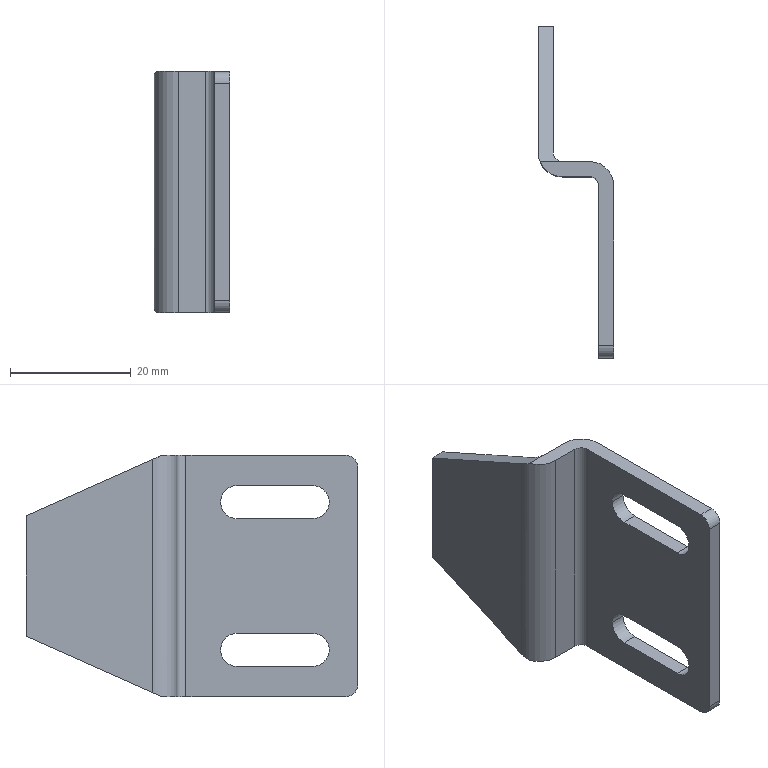Part | NX | features BREP 1 | 1 solid | 28 faces | box 12.5 x 55 x 40 mm | volume 5235 mm3 | plane 16 | cylinder 12 | commonest cylinder face diameters 5.5 x6 3 x2 4 x2 8 x2
STEP:
#1=CARTESIAN_POINT('',(0.,-7.25,-12.25));
#2=VERTEX_POINT('',#1);
#3=CARTESIAN_POINT('',(0.,-10.,-9.5));
#4=VERTEX_POINT('',#3);
#5=CARTESIAN_POINT('',(0.,-10.,-12.25));
#6=DIRECTION('',(1.,0.,0.));
#7=DIRECTION('',(0.,1.,0.));
#8=AXIS2_PLACEMENT_3D('',#5,#6,#7);
#9=CIRCLE('',#8,2.75);
#10=EDGE_CURVE('',#2,#4,#9,.T.);
#11=ORIENTED_EDGE('',*,*,#10,.F.);
#12=CARTESIAN_POINT('',(2.5,-7.25,-12.25));
#13=VERTEX_POINT('',#12);
#14=CARTESIAN_POINT('',(-10.,-7.25,-12.25));
#15=DIRECTION('',(1.,0.,0.));
#16=VECTOR('',#15,1000.);
#17=LINE('',#14,#16);
#18=EDGE_CURVE('',#2,#13,#17,.T.);
#19=ORIENTED_EDGE('',*,*,#18,.T.);
#20=CARTESIAN_POINT('',(2.5,-10.,-9.5));
#21=VERTEX_POINT('',#20);
#22=CARTESIAN_POINT('',(2.5,-10.,-12.25));
#23=DIRECTION('',(1.,0.,0.));
#24=DIRECTION('',(0.,-1.,0.));
#25=AXIS2_PLACEMENT_3D('',#22,#23,#24);
#26=CIRCLE('',#25,2.75);
#27=EDGE_CURVE('',#13,#21,#26,.T.);
#28=ORIENTED_EDGE('',*,*,#27,.T.);
#29=CARTESIAN_POINT('',(-10.,-10.,-9.5));
#30=DIRECTION('',(1.,0.,0.));
#31=VECTOR('',#30,1000.);
#32=LINE('',#29,#31);
#33=EDGE_CURVE('',#4,#21,#32,.T.);
#34=ORIENTED_EDGE('',*,*,#33,.F.);
#35=EDGE_LOOP('',(#11,#19,#28,#34));
#36=FACE_BOUND('',#35,.T.);
#37=CARTESIAN_POINT('',(-10.,-10.,-12.25));
#38=DIRECTION('',(1.,0.,0.));
#39=DIRECTION('',(0.,1.,0.));
#40=AXIS2_PLACEMENT_3D('',#37,#38,#39);
#41=CYLINDRICAL_SURFACE('',#40,2.75);
#42=ADVANCED_FACE('',(#36),#41,.F.);
#43=CARTESIAN_POINT('',(0.,-7.25,12.25));
#44=VERTEX_POINT('',#43);
#45=CARTESIAN_POINT('',(0.,-10.,15.));
#46=VERTEX_POINT('',#45);
#47=CARTESIAN_POINT('',(0.,-10.,12.25));
#48=DIRECTION('',(1.,0.,0.));
#49=DIRECTION('',(0.,1.,0.));
#50=AXIS2_PLACEMENT_3D('',#47,#48,#49);
#51=CIRCLE('',#50,2.75);
#52=EDGE_CURVE('',#44,#46,#51,.T.);
#53=ORIENTED_EDGE('',*,*,#52,.F.);
#54=CARTESIAN_POINT('',(2.5,-7.25,12.25));
#55=VERTEX_POINT('',#54);
#56=CARTESIAN_POINT('',(-10.,-7.25,12.25));
#57=DIRECTION('',(1.,0.,0.));
#58=VECTOR('',#57,1000.);
#59=LINE('',#56,#58);
#60=EDGE_CURVE('',#44,#55,#59,.T.);
#61=ORIENTED_EDGE('',*,*,#60,.T.);
#62=CARTESIAN_POINT('',(2.5,-10.,15.));
#63=VERTEX_POINT('',#62);
#64=CARTESIAN_POINT('',(2.5,-10.,12.25));
#65=DIRECTION('',(1.,0.,0.));
#66=DIRECTION('',(0.,1.,0.));
#67=AXIS2_PLACEMENT_3D('',#64,#65,#66);
#68=CIRCLE('',#67,2.75);
#69=EDGE_CURVE('',#55,#63,#68,.T.);
#70=ORIENTED_EDGE('',*,*,#69,.T.);
#71=CARTESIAN_POINT('',(-10.,-10.,15.));
#72=DIRECTION('',(1.,0.,0.));
#73=VECTOR('',#72,1000.);
#74=LINE('',#71,#73);
#75=EDGE_CURVE('',#46,#63,#74,.T.);
#76=ORIENTED_EDGE('',*,*,#75,.F.);
#77=EDGE_LOOP('',(#53,#61,#70,#76));
#78=FACE_BOUND('',#77,.T.);
#79=CARTESIAN_POINT('',(-10.,-10.,12.25));
#80=DIRECTION('',(1.,0.,0.));
#81=DIRECTION('',(0.,1.,0.));
#82=AXIS2_PLACEMENT_3D('',#79,#80,#81);
#83=CYLINDRICAL_SURFACE('',#82,2.75);
#84=ADVANCED_FACE('',(#78),#83,.F.);
#85=CARTESIAN_POINT('',(2.5,-30.,18.));
#86=VERTEX_POINT('',#85);
#87=CARTESIAN_POINT('',(2.5,-30.,-18.));
#88=VERTEX_POINT('',#87);
#89=CARTESIAN_POINT('',(2.5,-30.,20.));
#90=DIRECTION('',(0.,0.,-1.));
#91=VECTOR('',#90,1000.);
#92=LINE('',#89,#91);
#93=EDGE_CURVE('',#86,#88,#92,.T.);
#94=ORIENTED_EDGE('',*,*,#93,.T.);
#95=CARTESIAN_POINT('',(2.5,-28.,-20.));
#96=VERTEX_POINT('',#95);
#97=CARTESIAN_POINT('',(2.5,-28.,-18.));
#98=DIRECTION('',(1.,0.,0.));
#99=DIRECTION('',(0.,-1.,0.));
#100=AXIS2_PLACEMENT_3D('',#97,#98,#99);
#101=CIRCLE('',#100,2.);
#102=EDGE_CURVE('',#88,#96,#101,.T.);
#103=ORIENTED_EDGE('',*,*,#102,.T.);
#104=CARTESIAN_POINT('',(2.5,-1.5,-20.));
#105=VERTEX_POINT('',#104);
#106=CARTESIAN_POINT('',(2.5,2.5,-20.));
#107=DIRECTION('',(0.,1.,0.));
#108=VECTOR('',#107,1000.);
#109=LINE('',#106,#108);
#110=EDGE_CURVE('',#96,#105,#109,.T.);
#111=ORIENTED_EDGE('',*,*,#110,.T.);
#112=CARTESIAN_POINT('',(2.5,-1.5,20.));
#113=VERTEX_POINT('',#112);
#114=CARTESIAN_POINT('',(2.5,-1.5,20.));
#115=DIRECTION('',(0.,0.,1.));
#116=VECTOR('',#115,1000.);
#117=LINE('',#114,#116);
#118=EDGE_CURVE('',#105,#113,#117,.T.);
#119=ORIENTED_EDGE('',*,*,#118,.T.);
#120=CARTESIAN_POINT('',(2.5,-28.,20.));
#121=VERTEX_POINT('',#120);
#122=CARTESIAN_POINT('',(2.5,2.5,20.));
#123=DIRECTION('',(0.,1.,0.));
#124=VECTOR('',#123,1000.);
#125=LINE('',#122,#124);
#126=EDGE_CURVE('',#121,#113,#125,.T.);
#127=ORIENTED_EDGE('',*,*,#126,.F.);
#128=CARTESIAN_POINT('',(2.5,-28.,18.));
#129=DIRECTION('',(1.,0.,0.));
#130=DIRECTION('',(0.,-1.,0.));
#131=AXIS2_PLACEMENT_3D('',#128,#129,#130);
#132=CIRCLE('',#131,2.);
#133=EDGE_CURVE('',#121,#86,#132,.T.);
#134=ORIENTED_EDGE('',*,*,#133,.T.);
#135=EDGE_LOOP('',(#94,#103,#111,#119,#127,#134));
#136=FACE_BOUND('',#135,.T.);
#137=CARTESIAN_POINT('',(2.5,-22.5,-9.5));
#138=VERTEX_POINT('',#137);
#139=CARTESIAN_POINT('',(2.5,-10.,-9.5));
#140=DIRECTION('',(0.,-1.,0.));
#141=VECTOR('',#140,1000.);
#142=LINE('',#139,#141);
#143=EDGE_CURVE('',#21,#138,#142,.T.);
#144=ORIENTED_EDGE('',*,*,#143,.F.);
#145=ORIENTED_EDGE('',*,*,#27,.F.);
#146=CARTESIAN_POINT('',(2.5,-10.,-15.));
#147=VERTEX_POINT('',#146);
#148=CARTESIAN_POINT('',(2.5,-10.,-12.25));
#149=DIRECTION('',(1.,0.,0.));
#150=DIRECTION('',(0.,-1.,0.));
#151=AXIS2_PLACEMENT_3D('',#148,#149,#150);
#152=CIRCLE('',#151,2.75);
#153=EDGE_CURVE('',#147,#13,#152,.T.);
#154=ORIENTED_EDGE('',*,*,#153,.F.);
#155=CARTESIAN_POINT('',(2.5,-22.5,-15.));
#156=VERTEX_POINT('',#155);
#157=CARTESIAN_POINT('',(2.5,-10.,-15.));
#158=DIRECTION('',(0.,1.,0.));
#159=VECTOR('',#158,1000.);
#160=LINE('',#157,#159);
#161=EDGE_CURVE('',#156,#147,#160,.T.);
#162=ORIENTED_EDGE('',*,*,#161,.F.);
#163=CARTESIAN_POINT('',(2.5,-22.5,-12.25));
#164=DIRECTION('',(1.,0.,0.));
#165=DIRECTION('',(0.,-1.,0.));
#166=AXIS2_PLACEMENT_3D('',#163,#164,#165);
#167=CIRCLE('',#166,2.75);
#168=EDGE_CURVE('',#138,#156,#167,.T.);
#169=ORIENTED_EDGE('',*,*,#168,.F.);
#170=EDGE_LOOP('',(#144,#145,#154,#162,#169));
#171=FACE_BOUND('',#170,.T.);
#172=CARTESIAN_POINT('',(2.5,-22.5,15.));
#173=VERTEX_POINT('',#172);
#174=CARTESIAN_POINT('',(2.5,-10.,15.));
#175=DIRECTION('',(0.,-1.,0.));
#176=VECTOR('',#175,1000.);
#177=LINE('',#174,#176);
#178=EDGE_CURVE('',#63,#173,#177,.T.);
#179=ORIENTED_EDGE('',*,*,#178,.F.);
#180=ORIENTED_EDGE('',*,*,#69,.F.);
#181=CARTESIAN_POINT('',(2.5,-10.,9.5));
#182=VERTEX_POINT('',#181);
#183=CARTESIAN_POINT('',(2.5,-10.,12.25));
#184=DIRECTION('',(1.,0.,0.));
#185=DIRECTION('',(0.,1.,0.));
#186=AXIS2_PLACEMENT_3D('',#183,#184,#185);
#187=CIRCLE('',#186,2.75);
#188=EDGE_CURVE('',#182,#55,#187,.T.);
#189=ORIENTED_EDGE('',*,*,#188,.F.);
#190=CARTESIAN_POINT('',(2.5,-22.5,9.5));
#191=VERTEX_POINT('',#190);
#192=CARTESIAN_POINT('',(2.5,-10.,9.5));
#193=DIRECTION('',(0.,1.,0.));
#194=VECTOR('',#193,1000.);
#195=LINE('',#192,#194);
#196=EDGE_CURVE('',#191,#182,#195,.T.);
#197=ORIENTED_EDGE('',*,*,#196,.F.);
#198=CARTESIAN_POINT('',(2.5,-22.5,12.25));
#199=DIRECTION('',(1.,0.,0.));
#200=DIRECTION('',(0.,1.,0.));
#201=AXIS2_PLACEMENT_3D('',#198,#199,#200);
#202=CIRCLE('',#201,2.75);
#203=EDGE_CURVE('',#173,#191,#202,.T.);
#204=ORIENTED_EDGE('',*,*,#203,.F.);
#205=EDGE_LOOP('',(#179,#180,#189,#197,#204));
#206=FACE_BOUND('',#205,.T.);
#207=CARTESIAN_POINT('',(2.5,2.5,20.));
#208=DIRECTION('',(-1.,0.,0.));
#209=DIRECTION('',(0.,1.,0.));
#210=AXIS2_PLACEMENT_3D('',#207,#208,#209);
#211=PLANE('',#210);
#212=ADVANCED_FACE('',(#136,#171,#206),#211,.F.);
#213=CARTESIAN_POINT('',(-1.5,2.5,20.));
#214=VERTEX_POINT('',#213);
#215=CARTESIAN_POINT('',(-6.,2.5,20.));
#216=VERTEX_POINT('',#215);
#217=CARTESIAN_POINT('',(-7.5,2.5,20.));
#218=DIRECTION('',(-1.,0.,0.));
#219=VECTOR('',#218,1000.);
#220=LINE('',#217,#219);
#221=EDGE_CURVE('',#214,#216,#220,.T.);
#222=ORIENTED_EDGE('',*,*,#221,.F.);
#223=CARTESIAN_POINT('',(-1.5,2.5,-20.));
#224=VERTEX_POINT('',#223);
#225=CARTESIAN_POINT('',(-1.5,2.5,20.));
#226=DIRECTION('',(0.,0.,-1.));
#227=VECTOR('',#226,1000.);
#228=LINE('',#225,#227);
#229=EDGE_CURVE('',#214,#224,#228,.T.);
#230=ORIENTED_EDGE('',*,*,#229,.T.);
#231=CARTESIAN_POINT('',(-6.,2.5,-20.));
#232=VERTEX_POINT('',#231);
#233=CARTESIAN_POINT('',(-7.5,2.5,-20.));
#234=DIRECTION('',(-1.,0.,0.));
#235=VECTOR('',#234,1000.);
#236=LINE('',#233,#235);
#237=EDGE_CURVE('',#224,#232,#236,.T.);
#238=ORIENTED_EDGE('',*,*,#237,.T.);
#239=CARTESIAN_POINT('',(-6.,2.5,20.));
#240=DIRECTION('',(0.,0.,1.));
#241=VECTOR('',#240,1000.);
#242=LINE('',#239,#241);
#243=EDGE_CURVE('',#232,#216,#242,.T.);
#244=ORIENTED_EDGE('',*,*,#243,.T.);
#245=EDGE_LOOP('',(#222,#230,#238,#244));
#246=FACE_BOUND('',#245,.T.);
#247=CARTESIAN_POINT('',(-7.5,2.5,20.));
#248=DIRECTION('',(0.,-1.,0.));
#249=DIRECTION('',(0.,0.,-1.));
#250=AXIS2_PLACEMENT_3D('',#247,#248,#249);
#251=PLANE('',#250);
#252=ADVANCED_FACE('',(#246),#251,.F.);
#253=CARTESIAN_POINT('',(-7.5,25.,10.));
#254=VERTEX_POINT('',#253);
#255=CARTESIAN_POINT('',(-7.5,4.,19.333));
#256=VERTEX_POINT('',#255);
#257=CARTESIAN_POINT('',(-7.5,21.289,11.649));
#258=DIRECTION('',(0.,-0.9138,0.4061));
#259=VECTOR('',#258,1000.);
#260=LINE('',#257,#259);
#261=EDGE_CURVE('',#254,#256,#260,.T.);
#262=ORIENTED_EDGE('',*,*,#261,.T.);
#263=CARTESIAN_POINT('',(-7.5,4.,-19.333));
#264=VERTEX_POINT('',#263);
#265=CARTESIAN_POINT('',(-7.5,4.,-20.));
#266=DIRECTION('',(0.,0.,-1.));
#267=VECTOR('',#266,1000.);
#268=LINE('',#265,#267);
#269=EDGE_CURVE('',#256,#264,#268,.T.);
#270=ORIENTED_EDGE('',*,*,#269,.T.);
#271=CARTESIAN_POINT('',(-7.5,25.,-10.));
#272=VERTEX_POINT('',#271);
#273=CARTESIAN_POINT('',(-7.5,36.134,-5.052));
#274=DIRECTION('',(0.,0.9138,0.4061));
#275=VECTOR('',#274,1000.);
#276=LINE('',#273,#275);
#277=EDGE_CURVE('',#264,#272,#276,.T.);
#278=ORIENTED_EDGE('',*,*,#277,.T.);
#279=CARTESIAN_POINT('',(-7.5,25.,20.));
#280=DIRECTION('',(0.,0.,-1.));
#281=VECTOR('',#280,1000.);
#282=LINE('',#279,#281);
#283=EDGE_CURVE('',#254,#272,#282,.T.);
#284=ORIENTED_EDGE('',*,*,#283,.F.);
#285=EDGE_LOOP('',(#262,#270,#278,#284));
#286=FACE_BOUND('',#285,.T.);
#287=CARTESIAN_POINT('',(-7.5,25.,20.));
#288=DIRECTION('',(-1.,0.,0.));
#289=DIRECTION('',(0.,1.,0.));
#290=AXIS2_PLACEMENT_3D('',#287,#288,#289);
#291=PLANE('',#290);
#292=ADVANCED_FACE('',(#286),#291,.F.);
#293=ORIENTED_EDGE('',*,*,#283,.T.);
#294=CARTESIAN_POINT('',(-10.,25.,-10.));
#295=VERTEX_POINT('',#294);
#296=CARTESIAN_POINT('',(-10.,25.,-10.));
#297=DIRECTION('',(1.,0.,0.));
#298=VECTOR('',#297,1000.);
#299=LINE('',#296,#298);
#300=EDGE_CURVE('',#295,#272,#299,.T.);
#301=ORIENTED_EDGE('',*,*,#300,.F.);
#302=CARTESIAN_POINT('',(-10.,25.,10.));
#303=VERTEX_POINT('',#302);
#304=CARTESIAN_POINT('',(-10.,25.,20.));
#305=DIRECTION('',(0.,0.,-1.));
#306=VECTOR('',#305,1000.);
#307=LINE('',#304,#306);
#308=EDGE_CURVE('',#303,#295,#307,.T.);
#309=ORIENTED_EDGE('',*,*,#308,.F.);
#310=CARTESIAN_POINT('',(-10.,25.,10.));
#311=DIRECTION('',(1.,0.,0.));
#312=VECTOR('',#311,1000.);
#313=LINE('',#310,#312);
#314=EDGE_CURVE('',#303,#254,#313,.T.);
#315=ORIENTED_EDGE('',*,*,#314,.T.);
#316=EDGE_LOOP('',(#293,#301,#309,#315));
#317=FACE_BOUND('',#316,.T.);
#318=CARTESIAN_POINT('',(-10.,25.,20.));
#319=DIRECTION('',(0.,-1.,0.));
#320=DIRECTION('',(0.,0.,-1.));
#321=AXIS2_PLACEMENT_3D('',#318,#319,#320);
#322=PLANE('',#321);
#323=ADVANCED_FACE('',(#317),#322,.F.);
#324=CARTESIAN_POINT('',(-10.,4.,-19.333));
#325=VERTEX_POINT('',#324);
#326=CARTESIAN_POINT('',(-10.,25.,-10.));
#327=DIRECTION('',(0.,-0.9138,-0.4061));
#328=VECTOR('',#327,1000.);
#329=LINE('',#326,#328);
#330=EDGE_CURVE('',#295,#325,#329,.T.);
#331=ORIENTED_EDGE('',*,*,#330,.T.);
#332=CARTESIAN_POINT('',(-10.,4.,19.333));
#333=VERTEX_POINT('',#332);
#334=CARTESIAN_POINT('',(-10.,4.,20.));
#335=DIRECTION('',(0.,0.,1.));
#336=VECTOR('',#335,1000.);
#337=LINE('',#334,#336);
#338=EDGE_CURVE('',#325,#333,#337,.T.);
#339=ORIENTED_EDGE('',*,*,#338,.T.);
#340=CARTESIAN_POINT('',(-10.,25.,10.));
#341=DIRECTION('',(0.,0.9138,-0.4061));
#342=VECTOR('',#341,1000.);
#343=LINE('',#340,#342);
#344=EDGE_CURVE('',#333,#303,#343,.T.);
#345=ORIENTED_EDGE('',*,*,#344,.T.);
#346=ORIENTED_EDGE('',*,*,#308,.T.);
#347=EDGE_LOOP('',(#331,#339,#345,#346));
#348=FACE_BOUND('',#347,.T.);
#349=CARTESIAN_POINT('',(-10.,0.,20.));
#350=DIRECTION('',(1.,0.,0.));
#351=DIRECTION('',(0.,1.,0.));
#352=AXIS2_PLACEMENT_3D('',#349,#350,#351);
#353=PLANE('',#352);
#354=ADVANCED_FACE('',(#348),#353,.F.);
#355=CARTESIAN_POINT('',(-6.,0.,20.));
#356=VERTEX_POINT('',#355);
#357=CARTESIAN_POINT('',(-1.5,0.,20.));
#358=VERTEX_POINT('',#357);
#359=CARTESIAN_POINT('',(0.,0.,20.));
#360=DIRECTION('',(1.,0.,0.));
#361=VECTOR('',#360,1000.);
#362=LINE('',#359,#361);
#363=EDGE_CURVE('',#356,#358,#362,.T.);
#364=ORIENTED_EDGE('',*,*,#363,.F.);
#365=CARTESIAN_POINT('',(-6.,0.,-20.));
#366=VERTEX_POINT('',#365);
#367=CARTESIAN_POINT('',(-6.,0.,20.));
#368=DIRECTION('',(0.,0.,-1.));
#369=VECTOR('',#368,1000.);
#370=LINE('',#367,#369);
#371=EDGE_CURVE('',#356,#366,#370,.T.);
#372=ORIENTED_EDGE('',*,*,#371,.T.);
#373=CARTESIAN_POINT('',(-1.5,0.,-20.));
#374=VERTEX_POINT('',#373);
#375=CARTESIAN_POINT('',(0.,0.,-20.));
#376=DIRECTION('',(1.,0.,0.));
#377=VECTOR('',#376,1000.);
#378=LINE('',#375,#377);
#379=EDGE_CURVE('',#366,#374,#378,.T.);
#380=ORIENTED_EDGE('',*,*,#379,.T.);
#381=CARTESIAN_POINT('',(-1.5,0.,20.));
#382=DIRECTION('',(0.,0.,1.));
#383=VECTOR('',#382,1000.);
#384=LINE('',#381,#383);
#385=EDGE_CURVE('',#374,#358,#384,.T.);
#386=ORIENTED_EDGE('',*,*,#385,.T.);
#387=EDGE_LOOP('',(#364,#372,#380,#386));
#388=FACE_BOUND('',#387,.T.);
#389=CARTESIAN_POINT('',(0.,0.,20.));
#390=DIRECTION('',(0.,1.,0.));
#391=DIRECTION('',(1.,0.,0.));
#392=AXIS2_PLACEMENT_3D('',#389,#390,#391);
#393=PLANE('',#392);
#394=ADVANCED_FACE('',(#388),#393,.F.);
#395=CARTESIAN_POINT('',(0.,-1.5,-20.));
#396=VERTEX_POINT('',#395);
#397=CARTESIAN_POINT('',(0.,-28.,-20.));
#398=VERTEX_POINT('',#397);
#399=CARTESIAN_POINT('',(0.,-30.,-20.));
#400=DIRECTION('',(0.,-1.,0.));
#401=VECTOR('',#400,1000.);
#402=LINE('',#399,#401);
#403=EDGE_CURVE('',#396,#398,#402,.T.);
#404=ORIENTED_EDGE('',*,*,#403,.T.);
#405=CARTESIAN_POINT('',(0.,-30.,-18.));
#406=VERTEX_POINT('',#405);
#407=CARTESIAN_POINT('',(0.,-28.,-18.));
#408=DIRECTION('',(-1.,0.,0.));
#409=DIRECTION('',(0.,1.,0.));
#410=AXIS2_PLACEMENT_3D('',#407,#408,#409);
#411=CIRCLE('',#410,2.);
#412=EDGE_CURVE('',#398,#406,#411,.T.);
#413=ORIENTED_EDGE('',*,*,#412,.T.);
#414=CARTESIAN_POINT('',(0.,-30.,18.));
#415=VERTEX_POINT('',#414);
#416=CARTESIAN_POINT('',(0.,-30.,20.));
#417=DIRECTION('',(0.,0.,-1.));
#418=VECTOR('',#417,1000.);
#419=LINE('',#416,#418);
#420=EDGE_CURVE('',#415,#406,#419,.T.);
#421=ORIENTED_EDGE('',*,*,#420,.F.);
#422=CARTESIAN_POINT('',(0.,-28.,20.));
#423=VERTEX_POINT('',#422);
#424=CARTESIAN_POINT('',(0.,-28.,18.));
#425=DIRECTION('',(-1.,0.,0.));
#426=DIRECTION('',(0.,1.,0.));
#427=AXIS2_PLACEMENT_3D('',#424,#425,#426);
#428=CIRCLE('',#427,2.);
#429=EDGE_CURVE('',#415,#423,#428,.T.);
#430=ORIENTED_EDGE('',*,*,#429,.T.);
#431=CARTESIAN_POINT('',(0.,-1.5,20.));
#432=VERTEX_POINT('',#431);
#433=CARTESIAN_POINT('',(0.,-30.,20.));
#434=DIRECTION('',(0.,-1.,0.));
#435=VECTOR('',#434,1000.);
#436=LINE('',#433,#435);
#437=EDGE_CURVE('',#432,#423,#436,.T.);
#438=ORIENTED_EDGE('',*,*,#437,.F.);
#439=CARTESIAN_POINT('',(0.,-1.5,-20.));
#440=DIRECTION('',(0.,0.,-1.));
#441=VECTOR('',#440,1000.);
#442=LINE('',#439,#441);
#443=EDGE_CURVE('',#432,#396,#442,.T.);
#444=ORIENTED_EDGE('',*,*,#443,.T.);
#445=EDGE_LOOP('',(#404,#413,#421,#430,#438,#444));
#446=FACE_BOUND('',#445,.T.);
#447=CARTESIAN_POINT('',(0.,-22.5,-15.));
#448=VERTEX_POINT('',#447);
#449=CARTESIAN_POINT('',(0.,-10.,-15.));
#450=VERTEX_POINT('',#449);
#451=CARTESIAN_POINT('',(0.,-30.,-15.));
#452=DIRECTION('',(0.,1.,0.));
#453=VECTOR('',#452,1000.);
#454=LINE('',#451,#453);
#455=EDGE_CURVE('',#448,#450,#454,.T.);
#456=ORIENTED_EDGE('',*,*,#455,.T.);
#457=CARTESIAN_POINT('',(0.,-10.,-12.25));
#458=DIRECTION('',(1.,0.,0.));
#459=DIRECTION('',(0.,1.,0.));
#460=AXIS2_PLACEMENT_3D('',#457,#458,#459);
#461=CIRCLE('',#460,2.75);
#462=EDGE_CURVE('',#450,#2,#461,.T.);
#463=ORIENTED_EDGE('',*,*,#462,.T.);
#464=ORIENTED_EDGE('',*,*,#10,.T.);
#465=CARTESIAN_POINT('',(0.,-22.5,-9.5));
#466=VERTEX_POINT('',#465);
#467=CARTESIAN_POINT('',(0.,-30.,-9.5));
#468=DIRECTION('',(0.,-1.,0.));
#469=VECTOR('',#468,1000.);
#470=LINE('',#467,#469);
#471=EDGE_CURVE('',#4,#466,#470,.T.);
#472=ORIENTED_EDGE('',*,*,#471,.T.);
#473=CARTESIAN_POINT('',(0.,-22.5,-12.25));
#474=DIRECTION('',(1.,0.,0.));
#475=DIRECTION('',(0.,1.,0.));
#476=AXIS2_PLACEMENT_3D('',#473,#474,#475);
#477=CIRCLE('',#476,2.75);
#478=EDGE_CURVE('',#466,#448,#477,.T.);
#479=ORIENTED_EDGE('',*,*,#478,.T.);
#480=EDGE_LOOP('',(#456,#463,#464,#472,#479));
#481=FACE_BOUND('',#480,.T.);
#482=CARTESIAN_POINT('',(0.,-22.5,9.5));
#483=VERTEX_POINT('',#482);
#484=CARTESIAN_POINT('',(0.,-10.,9.5));
#485=VERTEX_POINT('',#484);
#486=CARTESIAN_POINT('',(0.,-30.,9.5));
#487=DIRECTION('',(0.,1.,0.));
#488=VECTOR('',#487,1000.);
#489=LINE('',#486,#488);
#490=EDGE_CURVE('',#483,#485,#489,.T.);
#491=ORIENTED_EDGE('',*,*,#490,.T.);
#492=CARTESIAN_POINT('',(0.,-10.,12.25));
#493=DIRECTION('',(1.,0.,0.));
#494=DIRECTION('',(0.,1.,0.));
#495=AXIS2_PLACEMENT_3D('',#492,#493,#494);
#496=CIRCLE('',#495,2.75);
#497=EDGE_CURVE('',#485,#44,#496,.T.);
#498=ORIENTED_EDGE('',*,*,#497,.T.);
#499=ORIENTED_EDGE('',*,*,#52,.T.);
#500=CARTESIAN_POINT('',(0.,-22.5,15.));
#501=VERTEX_POINT('',#500);
#502=CARTESIAN_POINT('',(0.,-30.,15.));
#503=DIRECTION('',(0.,-1.,0.));
#504=VECTOR('',#503,1000.);
#505=LINE('',#502,#504);
#506=EDGE_CURVE('',#46,#501,#505,.T.);
#507=ORIENTED_EDGE('',*,*,#506,.T.);
#508=CARTESIAN_POINT('',(0.,-22.5,12.25));
#509=DIRECTION('',(1.,0.,0.));
#510=DIRECTION('',(0.,1.,0.));
#511=AXIS2_PLACEMENT_3D('',#508,#509,#510);
#512=CIRCLE('',#511,2.75);
#513=EDGE_CURVE('',#501,#483,#512,.T.);
#514=ORIENTED_EDGE('',*,*,#513,.T.);
#515=EDGE_LOOP('',(#491,#498,#499,#507,#514));
#516=FACE_BOUND('',#515,.T.);
#517=CARTESIAN_POINT('',(0.,-30.,20.));
#518=DIRECTION('',(1.,0.,0.));
#519=DIRECTION('',(0.,1.,0.));
#520=AXIS2_PLACEMENT_3D('',#517,#518,#519);
#521=PLANE('',#520);
#522=ADVANCED_FACE('',(#446,#481,#516),#521,.F.);
#523=ORIENTED_EDGE('',*,*,#420,.T.);
#524=CARTESIAN_POINT('',(2.5,-30.,-18.));
#525=DIRECTION('',(1.,0.,0.));
#526=VECTOR('',#525,1000.);
#527=LINE('',#524,#526);
#528=EDGE_CURVE('',#406,#88,#527,.T.);
#529=ORIENTED_EDGE('',*,*,#528,.T.);
#530=ORIENTED_EDGE('',*,*,#93,.F.);
#531=CARTESIAN_POINT('',(2.5,-30.,18.));
#532=DIRECTION('',(-1.,0.,0.));
#533=VECTOR('',#532,1000.);
#534=LINE('',#531,#533);
#535=EDGE_CURVE('',#86,#415,#534,.T.);
#536=ORIENTED_EDGE('',*,*,#535,.T.);
#537=EDGE_LOOP('',(#523,#529,#530,#536));
#538=FACE_BOUND('',#537,.T.);
#539=CARTESIAN_POINT('',(2.5,-30.,20.));
#540=DIRECTION('',(0.,1.,0.));
#541=DIRECTION('',(1.,0.,0.));
#542=AXIS2_PLACEMENT_3D('',#539,#540,#541);
#543=PLANE('',#542);
#544=ADVANCED_FACE('',(#538),#543,.F.);
#545=ORIENTED_EDGE('',*,*,#437,.T.);
#546=CARTESIAN_POINT('',(0.,-28.,20.));
#547=DIRECTION('',(1.,0.,0.));
#548=VECTOR('',#547,1000.);
#549=LINE('',#546,#548);
#550=EDGE_CURVE('',#423,#121,#549,.T.);
#551=ORIENTED_EDGE('',*,*,#550,.T.);
#552=ORIENTED_EDGE('',*,*,#126,.T.);
#553=CARTESIAN_POINT('',(-1.5,-1.5,20.));
#554=DIRECTION('',(0.,0.,1.));
#555=DIRECTION('',(-1.,0.,0.));
#556=AXIS2_PLACEMENT_3D('',#553,#554,#555);
#557=CIRCLE('',#556,4.);
#558=EDGE_CURVE('',#113,#214,#557,.T.);
#559=ORIENTED_EDGE('',*,*,#558,.T.);
#560=ORIENTED_EDGE('',*,*,#221,.T.);
#561=CARTESIAN_POINT('',(-9.708,2.5,20.));
#562=VERTEX_POINT('',#561);
#563=CARTESIAN_POINT('',(-10.,2.5,20.));
#564=DIRECTION('',(1.,0.,0.));
#565=VECTOR('',#564,1000.);
#566=LINE('',#563,#565);
#567=EDGE_CURVE('',#562,#216,#566,.T.);
#568=ORIENTED_EDGE('',*,*,#567,.F.);
#569=CARTESIAN_POINT('',(-6.,4.,20.));
#570=DIRECTION('',(0.,0.,1.));
#571=DIRECTION('',(-1.,0.,0.));
#572=AXIS2_PLACEMENT_3D('',#569,#570,#571);
#573=CIRCLE('',#572,4.);
#574=EDGE_CURVE('',#562,#356,#573,.T.);
#575=ORIENTED_EDGE('',*,*,#574,.T.);
#576=ORIENTED_EDGE('',*,*,#363,.T.);
#577=CARTESIAN_POINT('',(-1.5,-1.5,20.));
#578=DIRECTION('',(0.,0.,-1.));
#579=DIRECTION('',(-1.,0.,0.));
#580=AXIS2_PLACEMENT_3D('',#577,#578,#579);
#581=CIRCLE('',#580,1.5);
#582=EDGE_CURVE('',#358,#432,#581,.T.);
#583=ORIENTED_EDGE('',*,*,#582,.T.);
#584=EDGE_LOOP('',(#545,#551,#552,#559,#560,#568,#575,#576,#583));
#585=FACE_BOUND('',#584,.T.);
#586=CARTESIAN_POINT('',(0.,0.,20.));
#587=DIRECTION('',(0.,0.,-1.));
#588=DIRECTION('',(0.,-1.,0.));
#589=AXIS2_PLACEMENT_3D('',#586,#587,#588);
#590=PLANE('',#589);
#591=ADVANCED_FACE('',(#585),#590,.F.);
#592=ORIENTED_EDGE('',*,*,#110,.F.);
#593=CARTESIAN_POINT('',(0.,-28.,-20.));
#594=DIRECTION('',(-1.,0.,0.));
#595=VECTOR('',#594,1000.);
#596=LINE('',#593,#595);
#597=EDGE_CURVE('',#96,#398,#596,.T.);
#598=ORIENTED_EDGE('',*,*,#597,.T.);
#599=ORIENTED_EDGE('',*,*,#403,.F.);
#600=CARTESIAN_POINT('',(-1.5,-1.5,-20.));
#601=DIRECTION('',(0.,0.,1.));
#602=DIRECTION('',(-1.,0.,0.));
#603=AXIS2_PLACEMENT_3D('',#600,#601,#602);
#604=CIRCLE('',#603,1.5);
#605=EDGE_CURVE('',#396,#374,#604,.T.);
#606=ORIENTED_EDGE('',*,*,#605,.T.);
#607=ORIENTED_EDGE('',*,*,#379,.F.);
#608=CARTESIAN_POINT('',(-9.708,2.5,-20.));
#609=VERTEX_POINT('',#608);
#610=CARTESIAN_POINT('',(-6.,4.,-20.));
#611=DIRECTION('',(0.,0.,-1.));
#612=DIRECTION('',(-1.,0.,0.));
#613=AXIS2_PLACEMENT_3D('',#610,#611,#612);
#614=CIRCLE('',#613,4.);
#615=EDGE_CURVE('',#366,#609,#614,.T.);
#616=ORIENTED_EDGE('',*,*,#615,.T.);
#617=CARTESIAN_POINT('',(-10.,2.5,-20.));
#618=DIRECTION('',(1.,0.,0.));
#619=VECTOR('',#618,1000.);
#620=LINE('',#617,#619);
#621=EDGE_CURVE('',#609,#232,#620,.T.);
#622=ORIENTED_EDGE('',*,*,#621,.T.);
#623=ORIENTED_EDGE('',*,*,#237,.F.);
#624=CARTESIAN_POINT('',(-1.5,-1.5,-20.));
#625=DIRECTION('',(0.,0.,-1.));
#626=DIRECTION('',(-1.,0.,0.));
#627=AXIS2_PLACEMENT_3D('',#624,#625,#626);
#628=CIRCLE('',#627,4.);
#629=EDGE_CURVE('',#224,#105,#628,.T.);
#630=ORIENTED_EDGE('',*,*,#629,.T.);
#631=EDGE_LOOP('',(#592,#598,#599,#606,#607,#616,#622,#623,#630));
#632=FACE_BOUND('',#631,.T.);
#633=CARTESIAN_POINT('',(0.,0.,-20.));
#634=DIRECTION('',(0.,0.,-1.));
#635=DIRECTION('',(0.,-1.,0.));
#636=AXIS2_PLACEMENT_3D('',#633,#634,#635);
#637=PLANE('',#636);
#638=ADVANCED_FACE('',(#632),#637,.T.);
#639=ORIENTED_EDGE('',*,*,#344,.F.);
#640=CARTESIAN_POINT('',(-10.,4.,19.333));
#641=CARTESIAN_POINT('',(-10.,3.484,19.563));
#642=CARTESIAN_POINT('',(-9.901,2.978,19.788));
#643=CARTESIAN_POINT('',(-9.708,2.5,20.));
#644=(BOUNDED_CURVE()B_SPLINE_CURVE(3,(#640,#641,#642,#643),.UNSPECIFIED.,.F.,.F.)B_SPLINE_CURVE_WITH_KNOTS((4,4),(1.571,1.955),.UNSPECIFIED.)CURVE()GEOMETRIC_REPRESENTATION_ITEM()RATIONAL_B_SPLINE_CURVE((1.,0.9877,0.9877,1.))REPRESENTATION_ITEM(''));
#645=EDGE_CURVE('',#333,#562,#644,.T.);
#646=ORIENTED_EDGE('',*,*,#645,.T.);
#647=ORIENTED_EDGE('',*,*,#567,.T.);
#648=CARTESIAN_POINT('',(-6.,2.5,20.));
#649=CARTESIAN_POINT('',(-6.879,2.5,20.));
#650=CARTESIAN_POINT('',(-7.5,3.121,19.724));
#651=CARTESIAN_POINT('',(-7.5,4.,19.333));
#652=(BOUNDED_CURVE()B_SPLINE_CURVE(3,(#648,#649,#650,#651),.UNSPECIFIED.,.F.,.F.)B_SPLINE_CURVE_WITH_KNOTS((4,4),(0.,1.571),.UNSPECIFIED.)CURVE()GEOMETRIC_REPRESENTATION_ITEM()RATIONAL_B_SPLINE_CURVE((1.,0.8047,0.8047,1.))REPRESENTATION_ITEM(''));
#653=EDGE_CURVE('',#216,#256,#652,.T.);
#654=ORIENTED_EDGE('',*,*,#653,.T.);
#655=ORIENTED_EDGE('',*,*,#261,.F.);
#656=ORIENTED_EDGE('',*,*,#314,.F.);
#657=EDGE_LOOP('',(#639,#646,#647,#654,#655,#656));
#658=FACE_BOUND('',#657,.T.);
#659=CARTESIAN_POINT('',(-10.,25.,10.));
#660=DIRECTION('',(0.,-0.4061,-0.9138));
#661=DIRECTION('',(0.,-0.9138,0.4061));
#662=AXIS2_PLACEMENT_3D('',#659,#660,#661);
#663=PLANE('',#662);
#664=ADVANCED_FACE('',(#658),#663,.F.);
#665=ORIENTED_EDGE('',*,*,#621,.F.);
#666=CARTESIAN_POINT('',(-9.708,2.5,-20.));
#667=CARTESIAN_POINT('',(-9.901,2.978,-19.788));
#668=CARTESIAN_POINT('',(-10.,3.484,-19.563));
#669=CARTESIAN_POINT('',(-10.,4.,-19.333));
#670=(BOUNDED_CURVE()B_SPLINE_CURVE(3,(#666,#667,#668,#669),.UNSPECIFIED.,.F.,.F.)B_SPLINE_CURVE_WITH_KNOTS((4,4),(1.186,1.571),.UNSPECIFIED.)CURVE()GEOMETRIC_REPRESENTATION_ITEM()RATIONAL_B_SPLINE_CURVE((1.,0.9877,0.9877,1.))REPRESENTATION_ITEM(''));
#671=EDGE_CURVE('',#609,#325,#670,.T.);
#672=ORIENTED_EDGE('',*,*,#671,.T.);
#673=ORIENTED_EDGE('',*,*,#330,.F.);
#674=ORIENTED_EDGE('',*,*,#300,.T.);
#675=ORIENTED_EDGE('',*,*,#277,.F.);
#676=CARTESIAN_POINT('',(-7.5,4.,-19.333));
#677=CARTESIAN_POINT('',(-7.5,3.121,-19.724));
#678=CARTESIAN_POINT('',(-6.879,2.5,-20.));
#679=CARTESIAN_POINT('',(-6.,2.5,-20.));
#680=(BOUNDED_CURVE()B_SPLINE_CURVE(3,(#676,#677,#678,#679),.UNSPECIFIED.,.F.,.F.)B_SPLINE_CURVE_WITH_KNOTS((4,4),(1.571,3.142),.UNSPECIFIED.)CURVE()GEOMETRIC_REPRESENTATION_ITEM()RATIONAL_B_SPLINE_CURVE((1.,0.8047,0.8047,1.))REPRESENTATION_ITEM(''));
#681=EDGE_CURVE('',#264,#232,#680,.T.);
#682=ORIENTED_EDGE('',*,*,#681,.T.);
#683=EDGE_LOOP('',(#665,#672,#673,#674,#675,#682));
#684=FACE_BOUND('',#683,.T.);
#685=CARTESIAN_POINT('',(-10.,25.,-10.));
#686=DIRECTION('',(0.,-0.4061,0.9138));
#687=DIRECTION('',(-1.,0.,0.));
#688=AXIS2_PLACEMENT_3D('',#685,#686,#687);
#689=PLANE('',#688);
#690=ADVANCED_FACE('',(#684),#689,.F.);
#691=ORIENTED_EDGE('',*,*,#60,.F.);
#692=ORIENTED_EDGE('',*,*,#497,.F.);
#693=CARTESIAN_POINT('',(-10.,-10.,9.5));
#694=DIRECTION('',(1.,0.,0.));
#695=VECTOR('',#694,1000.);
#696=LINE('',#693,#695);
#697=EDGE_CURVE('',#485,#182,#696,.T.);
#698=ORIENTED_EDGE('',*,*,#697,.T.);
#699=ORIENTED_EDGE('',*,*,#188,.T.);
#700=EDGE_LOOP('',(#691,#692,#698,#699));
#701=FACE_BOUND('',#700,.T.);
#702=CARTESIAN_POINT('',(-10.,-10.,12.25));
#703=DIRECTION('',(1.,0.,0.));
#704=DIRECTION('',(0.,1.,0.));
#705=AXIS2_PLACEMENT_3D('',#702,#703,#704);
#706=CYLINDRICAL_SURFACE('',#705,2.75);
#707=ADVANCED_FACE('',(#701),#706,.F.);
#708=CARTESIAN_POINT('',(-10.,-22.5,9.5));
#709=DIRECTION('',(1.,0.,0.));
#710=VECTOR('',#709,1000.);
#711=LINE('',#708,#710);
#712=EDGE_CURVE('',#483,#191,#711,.T.);
#713=ORIENTED_EDGE('',*,*,#712,.T.);
#714=ORIENTED_EDGE('',*,*,#196,.T.);
#715=ORIENTED_EDGE('',*,*,#697,.F.);
#716=ORIENTED_EDGE('',*,*,#490,.F.);
#717=EDGE_LOOP('',(#713,#714,#715,#716));
#718=FACE_BOUND('',#717,.T.);
#719=CARTESIAN_POINT('',(-10.,-10.,9.5));
#720=DIRECTION('',(0.,0.,-1.));
#721=DIRECTION('',(-1.,0.,0.));
#722=AXIS2_PLACEMENT_3D('',#719,#720,#721);
#723=PLANE('',#722);
#724=ADVANCED_FACE('',(#718),#723,.F.);
#725=CARTESIAN_POINT('',(-10.,-22.5,15.));
#726=DIRECTION('',(1.,0.,0.));
#727=VECTOR('',#726,1000.);
#728=LINE('',#725,#727);
#729=EDGE_CURVE('',#501,#173,#728,.T.);
#730=ORIENTED_EDGE('',*,*,#729,.T.);
#731=ORIENTED_EDGE('',*,*,#203,.T.);
#732=ORIENTED_EDGE('',*,*,#712,.F.);
#733=ORIENTED_EDGE('',*,*,#513,.F.);
#734=EDGE_LOOP('',(#730,#731,#732,#733));
#735=FACE_BOUND('',#734,.T.);
#736=CARTESIAN_POINT('',(-10.,-22.5,12.25));
#737=DIRECTION('',(1.,0.,0.));
#738=DIRECTION('',(0.,1.,0.));
#739=AXIS2_PLACEMENT_3D('',#736,#737,#738);
#740=CYLINDRICAL_SURFACE('',#739,2.75);
#741=ADVANCED_FACE('',(#735),#740,.F.);
#742=ORIENTED_EDGE('',*,*,#75,.T.);
#743=ORIENTED_EDGE('',*,*,#178,.T.);
#744=ORIENTED_EDGE('',*,*,#729,.F.);
#745=ORIENTED_EDGE('',*,*,#506,.F.);
#746=EDGE_LOOP('',(#742,#743,#744,#745));
#747=FACE_BOUND('',#746,.T.);
#748=CARTESIAN_POINT('',(-10.,-10.,15.));
#749=DIRECTION('',(0.,0.,1.));
#750=DIRECTION('',(1.,0.,0.));
#751=AXIS2_PLACEMENT_3D('',#748,#749,#750);
#752=PLANE('',#751);
#753=ADVANCED_FACE('',(#747),#752,.F.);
#754=ORIENTED_EDGE('',*,*,#18,.F.);
#755=ORIENTED_EDGE('',*,*,#462,.F.);
#756=CARTESIAN_POINT('',(-10.,-10.,-15.));
#757=DIRECTION('',(1.,0.,0.));
#758=VECTOR('',#757,1000.);
#759=LINE('',#756,#758);
#760=EDGE_CURVE('',#450,#147,#759,.T.);
#761=ORIENTED_EDGE('',*,*,#760,.T.);
#762=ORIENTED_EDGE('',*,*,#153,.T.);
#763=EDGE_LOOP('',(#754,#755,#761,#762));
#764=FACE_BOUND('',#763,.T.);
#765=CARTESIAN_POINT('',(-10.,-10.,-12.25));
#766=DIRECTION('',(1.,0.,0.));
#767=DIRECTION('',(0.,1.,0.));
#768=AXIS2_PLACEMENT_3D('',#765,#766,#767);
#769=CYLINDRICAL_SURFACE('',#768,2.75);
#770=ADVANCED_FACE('',(#764),#769,.F.);
#771=CARTESIAN_POINT('',(-10.,-22.5,-15.));
#772=DIRECTION('',(1.,0.,0.));
#773=VECTOR('',#772,1000.);
#774=LINE('',#771,#773);
#775=EDGE_CURVE('',#448,#156,#774,.T.);
#776=ORIENTED_EDGE('',*,*,#775,.T.);
#777=ORIENTED_EDGE('',*,*,#161,.T.);
#778=ORIENTED_EDGE('',*,*,#760,.F.);
#779=ORIENTED_EDGE('',*,*,#455,.F.);
#780=EDGE_LOOP('',(#776,#777,#778,#779));
#781=FACE_BOUND('',#780,.T.);
#782=CARTESIAN_POINT('',(-10.,-10.,-15.));
#783=DIRECTION('',(0.,0.,-1.));
#784=DIRECTION('',(0.,-1.,0.));
#785=AXIS2_PLACEMENT_3D('',#782,#783,#784);
#786=PLANE('',#785);
#787=ADVANCED_FACE('',(#781),#786,.F.);
#788=CARTESIAN_POINT('',(-10.,-22.5,-9.5));
#789=DIRECTION('',(1.,0.,0.));
#790=VECTOR('',#789,1000.);
#791=LINE('',#788,#790);
#792=EDGE_CURVE('',#466,#138,#791,.T.);
#793=ORIENTED_EDGE('',*,*,#792,.T.);
#794=ORIENTED_EDGE('',*,*,#168,.T.);
#795=ORIENTED_EDGE('',*,*,#775,.F.);
#796=ORIENTED_EDGE('',*,*,#478,.F.);
#797=EDGE_LOOP('',(#793,#794,#795,#796));
#798=FACE_BOUND('',#797,.T.);
#799=CARTESIAN_POINT('',(-10.,-22.5,-12.25));
#800=DIRECTION('',(1.,0.,0.));
#801=DIRECTION('',(0.,1.,0.));
#802=AXIS2_PLACEMENT_3D('',#799,#800,#801);
#803=CYLINDRICAL_SURFACE('',#802,2.75);
#804=ADVANCED_FACE('',(#798),#803,.F.);
#805=ORIENTED_EDGE('',*,*,#33,.T.);
#806=ORIENTED_EDGE('',*,*,#143,.T.);
#807=ORIENTED_EDGE('',*,*,#792,.F.);
#808=ORIENTED_EDGE('',*,*,#471,.F.);
#809=EDGE_LOOP('',(#805,#806,#807,#808));
#810=FACE_BOUND('',#809,.T.);
#811=CARTESIAN_POINT('',(-10.,-10.,-9.5));
#812=DIRECTION('',(0.,0.,1.));
#813=DIRECTION('',(0.,-1.,0.));
#814=AXIS2_PLACEMENT_3D('',#811,#812,#813);
#815=PLANE('',#814);
#816=ADVANCED_FACE('',(#810),#815,.F.);
#817=ORIENTED_EDGE('',*,*,#412,.F.);
#818=ORIENTED_EDGE('',*,*,#597,.F.);
#819=ORIENTED_EDGE('',*,*,#102,.F.);
#820=ORIENTED_EDGE('',*,*,#528,.F.);
#821=EDGE_LOOP('',(#817,#818,#819,#820));
#822=FACE_BOUND('',#821,.T.);
#823=CARTESIAN_POINT('',(2.5,-28.,-18.));
#824=DIRECTION('',(-1.,0.,0.));
#825=DIRECTION('',(0.,0.,1.));
#826=AXIS2_PLACEMENT_3D('',#823,#824,#825);
#827=CYLINDRICAL_SURFACE('',#826,2.);
#828=ADVANCED_FACE('',(#822),#827,.T.);
#829=ORIENTED_EDGE('',*,*,#429,.F.);
#830=ORIENTED_EDGE('',*,*,#535,.F.);
#831=ORIENTED_EDGE('',*,*,#133,.F.);
#832=ORIENTED_EDGE('',*,*,#550,.F.);
#833=EDGE_LOOP('',(#829,#830,#831,#832));
#834=FACE_BOUND('',#833,.T.);
#835=CARTESIAN_POINT('',(0.,-28.,18.));
#836=DIRECTION('',(1.,0.,0.));
#837=DIRECTION('',(0.,0.,-1.));
#838=AXIS2_PLACEMENT_3D('',#835,#836,#837);
#839=CYLINDRICAL_SURFACE('',#838,2.);
#840=ADVANCED_FACE('',(#834),#839,.T.);
#841=ORIENTED_EDGE('',*,*,#645,.F.);
#842=ORIENTED_EDGE('',*,*,#338,.F.);
#843=ORIENTED_EDGE('',*,*,#671,.F.);
#844=ORIENTED_EDGE('',*,*,#615,.F.);
#845=ORIENTED_EDGE('',*,*,#371,.F.);
#846=ORIENTED_EDGE('',*,*,#574,.F.);
#847=EDGE_LOOP('',(#841,#842,#843,#844,#845,#846));
#848=FACE_BOUND('',#847,.T.);
#849=CARTESIAN_POINT('',(-6.,4.,20.));
#850=DIRECTION('',(0.,0.,-1.));
#851=DIRECTION('',(-1.,0.,0.));
#852=AXIS2_PLACEMENT_3D('',#849,#850,#851);
#853=CYLINDRICAL_SURFACE('',#852,4.);
#854=ADVANCED_FACE('',(#848),#853,.T.);
#855=ORIENTED_EDGE('',*,*,#558,.F.);
#856=ORIENTED_EDGE('',*,*,#118,.F.);
#857=ORIENTED_EDGE('',*,*,#629,.F.);
#858=ORIENTED_EDGE('',*,*,#229,.F.);
#859=EDGE_LOOP('',(#855,#856,#857,#858));
#860=FACE_BOUND('',#859,.T.);
#861=CARTESIAN_POINT('',(-1.5,-1.5,20.));
#862=DIRECTION('',(0.,0.,-1.));
#863=DIRECTION('',(-1.,0.,0.));
#864=AXIS2_PLACEMENT_3D('',#861,#862,#863);
#865=CYLINDRICAL_SURFACE('',#864,4.);
#866=ADVANCED_FACE('',(#860),#865,.T.);
#867=ORIENTED_EDGE('',*,*,#653,.F.);
#868=ORIENTED_EDGE('',*,*,#243,.F.);
#869=ORIENTED_EDGE('',*,*,#681,.F.);
#870=ORIENTED_EDGE('',*,*,#269,.F.);
#871=EDGE_LOOP('',(#867,#868,#869,#870));
#872=FACE_BOUND('',#871,.T.);
#873=CARTESIAN_POINT('',(-6.,4.,20.));
#874=DIRECTION('',(0.,0.,1.));
#875=DIRECTION('',(1.,0.,0.));
#876=AXIS2_PLACEMENT_3D('',#873,#874,#875);
#877=CYLINDRICAL_SURFACE('',#876,1.5);
#878=ADVANCED_FACE('',(#872),#877,.F.);
#879=ORIENTED_EDGE('',*,*,#582,.F.);
#880=ORIENTED_EDGE('',*,*,#385,.F.);
#881=ORIENTED_EDGE('',*,*,#605,.F.);
#882=ORIENTED_EDGE('',*,*,#443,.F.);
#883=EDGE_LOOP('',(#879,#880,#881,#882));
#884=FACE_BOUND('',#883,.T.);
#885=CARTESIAN_POINT('',(-1.5,-1.5,20.));
#886=DIRECTION('',(0.,0.,1.));
#887=DIRECTION('',(1.,0.,0.));
#888=AXIS2_PLACEMENT_3D('',#885,#886,#887);
#889=CYLINDRICAL_SURFACE('',#888,1.5);
#890=ADVANCED_FACE('',(#884),#889,.F.);
#891=CLOSED_SHELL('',(#42,#84,#212,#252,#292,#323,#354,#394,#522,#544,#591,#638,#664,#690,#707,#724,#741,#753,#770,#787,#804,#816,#828,#840,#854,#866,#878,#890));
#892=MANIFOLD_SOLID_BREP('',#891);
#893=(LENGTH_UNIT()NAMED_UNIT(*)SI_UNIT(.MILLI.,.METRE.));
#894=UNCERTAINTY_MEASURE_WITH_UNIT(LENGTH_MEASURE(0.00001),#893,'','');
#895=(NAMED_UNIT(*)PLANE_ANGLE_UNIT()SI_UNIT($,.RADIAN.));
#896=(NAMED_UNIT(*)SI_UNIT($,.STERADIAN.)SOLID_ANGLE_UNIT());
#897=(GEOMETRIC_REPRESENTATION_CONTEXT(3)GLOBAL_UNCERTAINTY_ASSIGNED_CONTEXT((#894))GLOBAL_UNIT_ASSIGNED_CONTEXT((#893,#895,#896))REPRESENTATION_CONTEXT('',''));
#898=ADVANCED_BREP_SHAPE_REPRESENTATION('',(#892),#897);